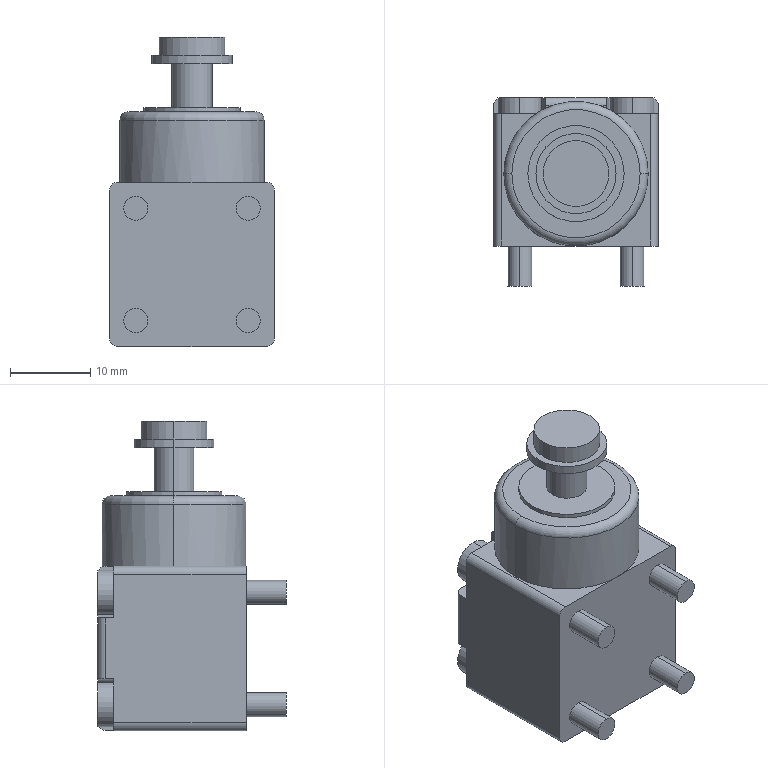Part | SolidWorks | features BaseBody 1 | 1 solid | 76 faces | box 20.5 x 23.5 x 38.55 mm | volume 10352 mm3 | cylinder 38 | plane 36 | torus 2 | commonest cylinder face diameters 2 x8 3 x8 5.5 x8 6.4 x4 5 x2 8.2 x2